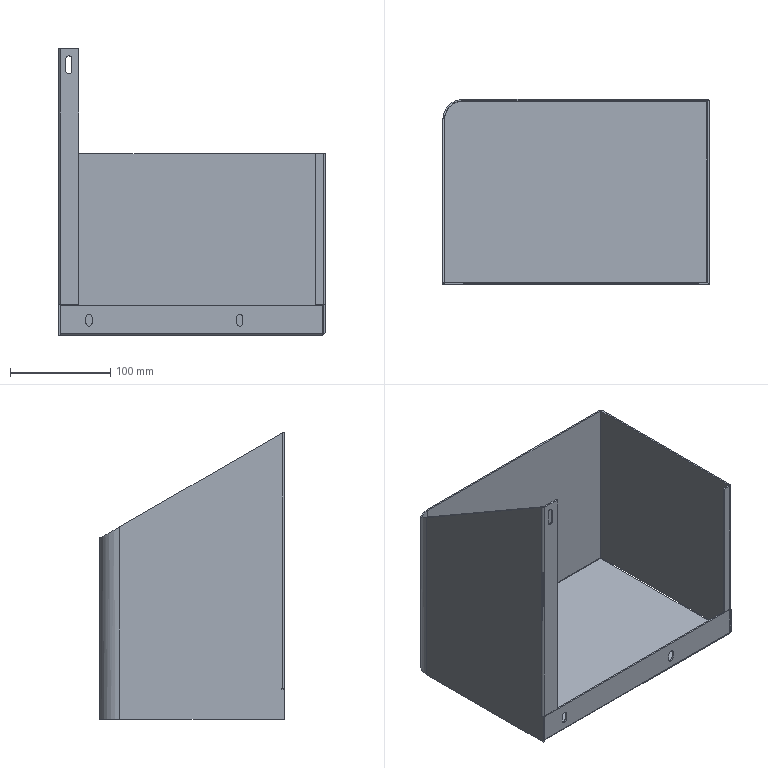Part | SolidWorks | features ICE 5, EdgeFlange 2, SMBaseFlange 2, SMMiteredFlange 2, FlatPattern 1, LPattern 1, SheetMetal 1 | 1 solid | 85 faces | box 265 x 184 x 285 mm | volume 272700 mm3 | plane 60 | cylinder 22 | spline 3 | commonest cylinder face diameters 6 x9 1 x5 4 x5 36.6 x1 37 x1 40 x1